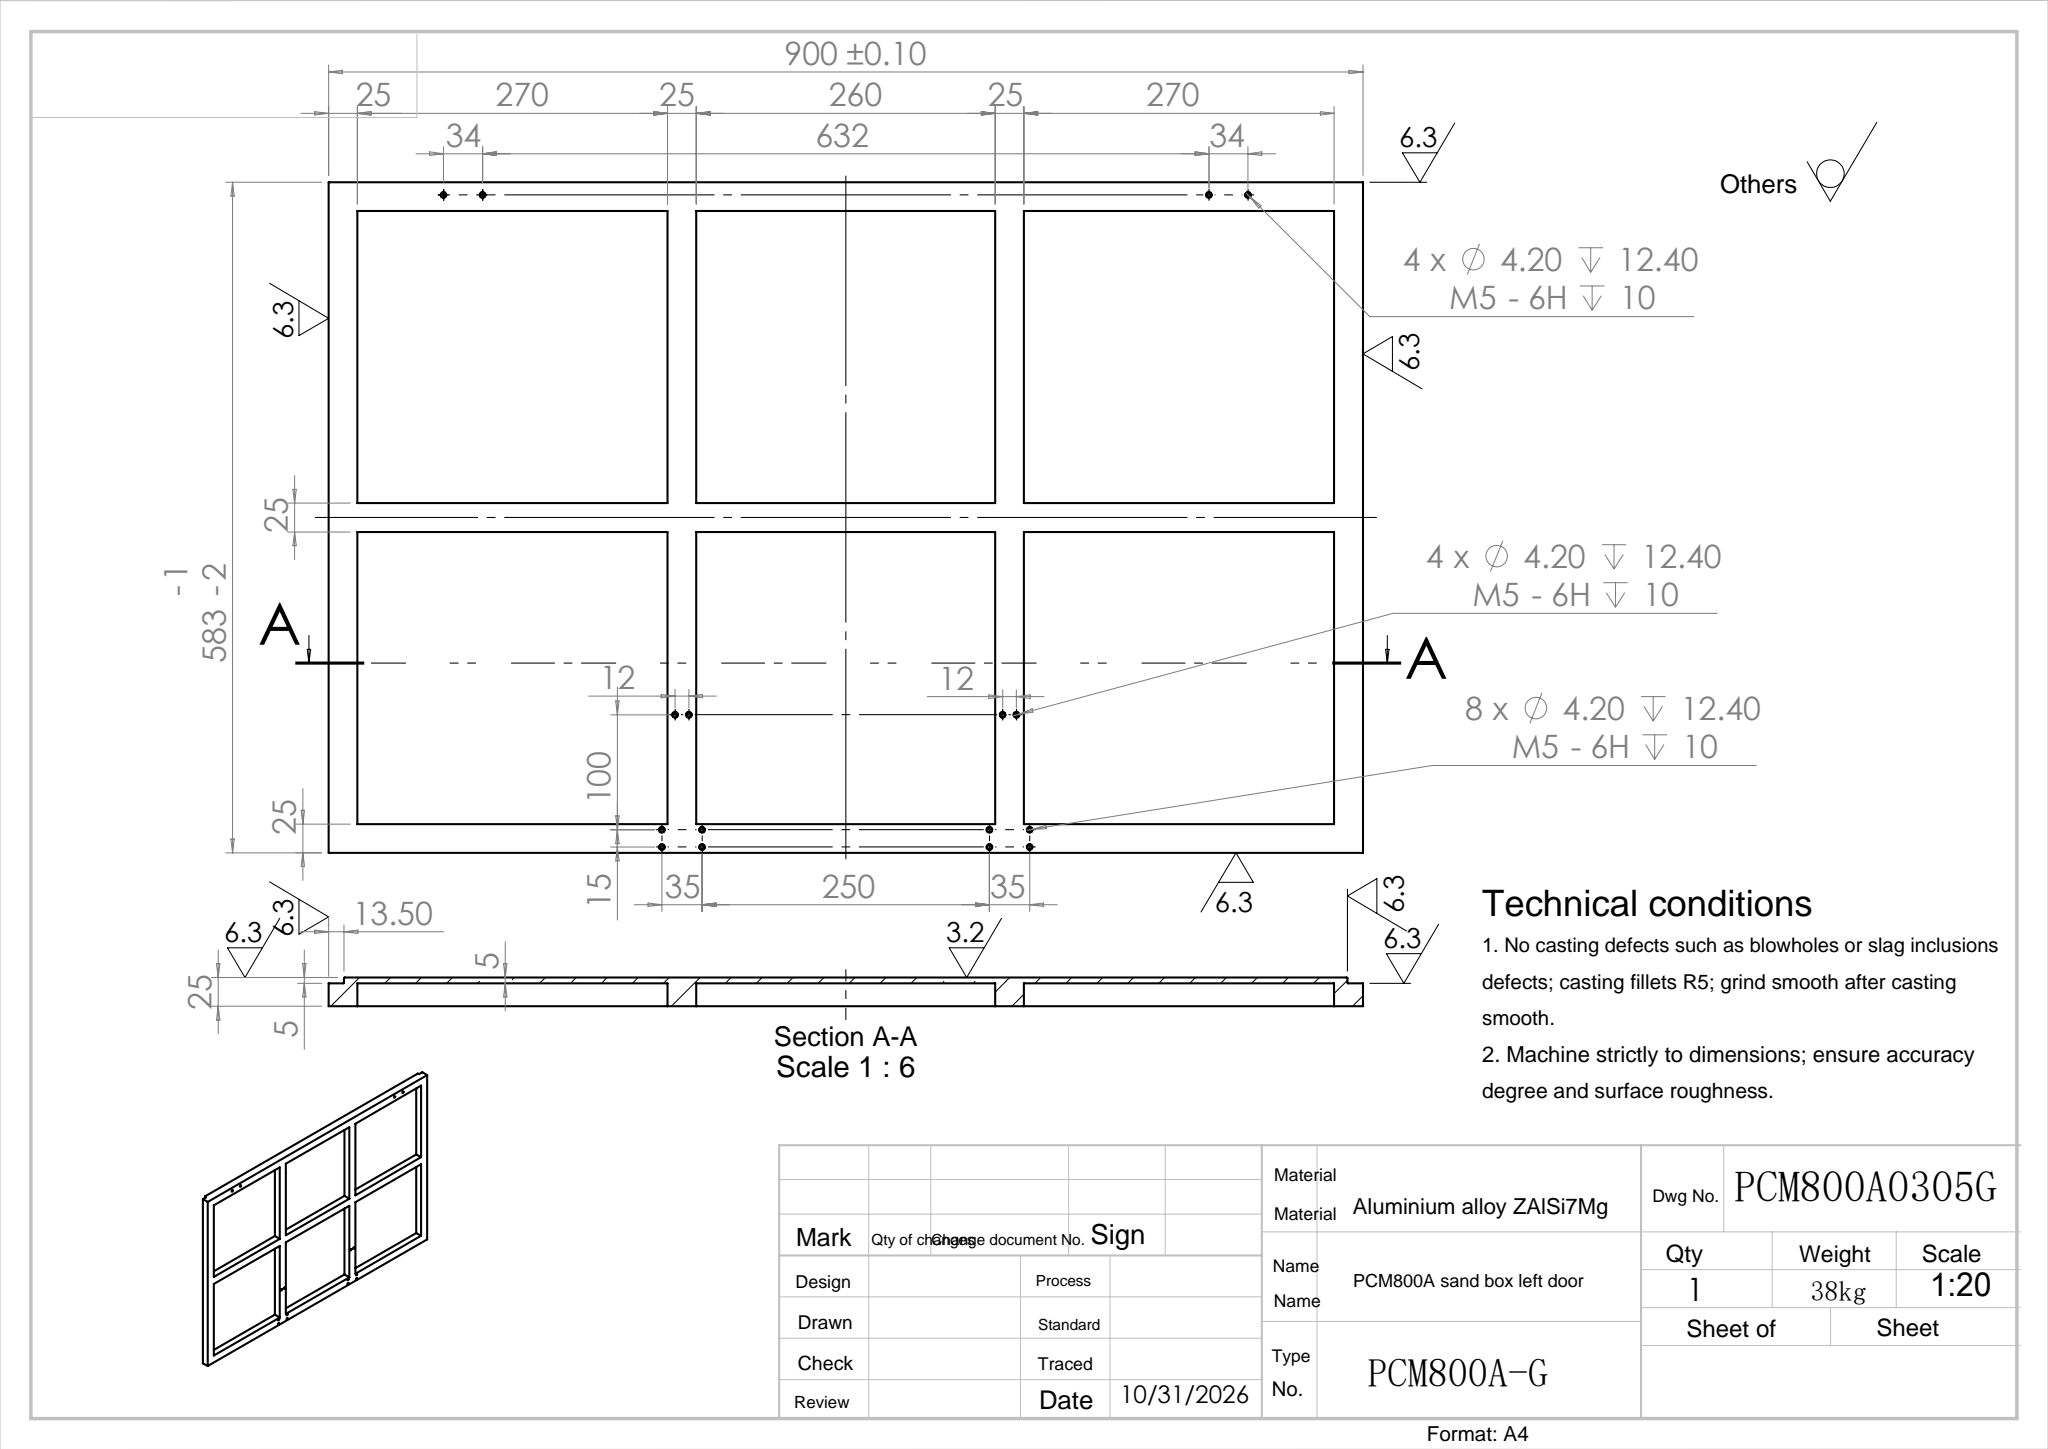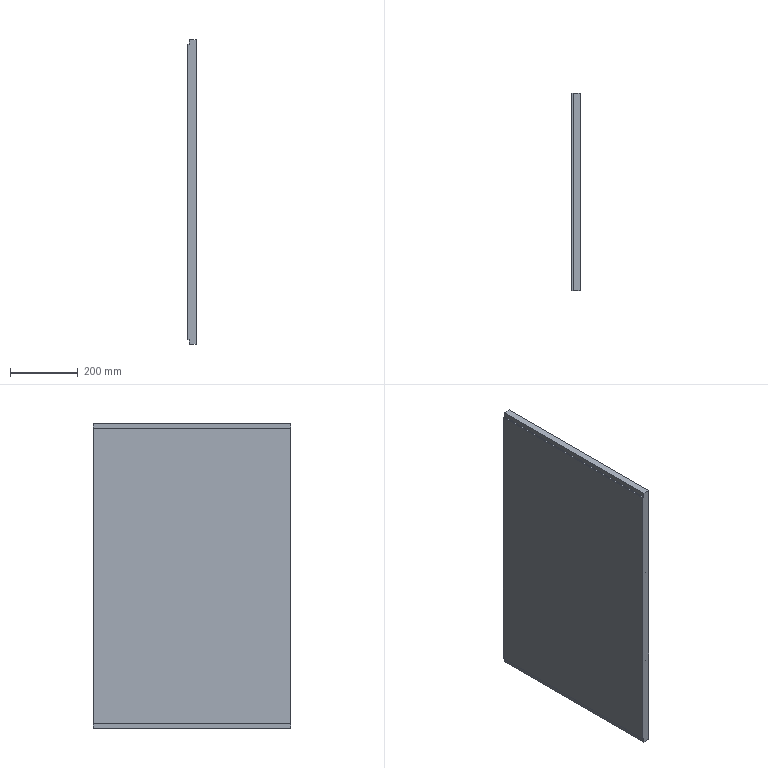Part | SolidWorks | features Boss 4, 3DProfileFeature 3, HoleWzd 3, LPattern 3, Chamfer 2, Cut 2, Extrusion 1 | 1 solid | 156 faces | box 25 x 583 x 900 mm | volume 4907028 mm3 | cylinder 64 | plane 60 | cone 32 | commonest cylinder face diameters 4.2 x32 5 x32